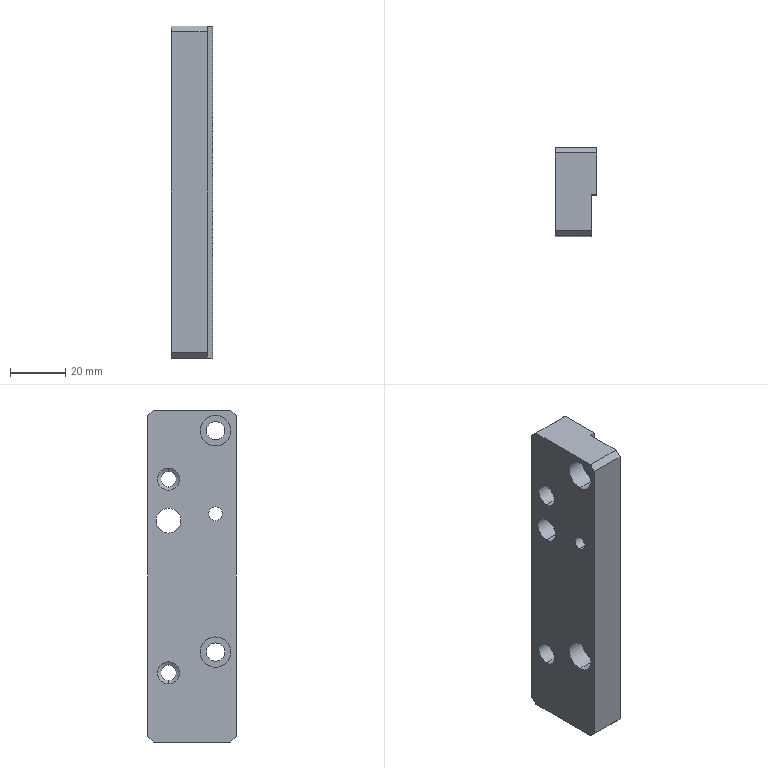Part | SolidWorks | features HoleWzd 5, Chamfer 1, Cut 1, Extrusion 1 | 1 solid | 44 faces | box 15 x 32 x 120 mm | volume 49288 mm3 | cylinder 24 | plane 16 | cone 4 | commonest cylinder face diameters 5.5 x4 6.6 x4 8 x4 10 x4 11 x4 5 x2
STEP:
#1=CARTESIAN_POINT('',(13.,-8.5,20.));
#2=VERTEX_POINT('',#1);
#3=CARTESIAN_POINT('',(13.,-8.5,25.));
#4=VERTEX_POINT('',#3);
#5=CARTESIAN_POINT('',(13.,-8.5,22.5));
#6=DIRECTION('',(-1.,0.,0.));
#7=DIRECTION('',(0.,0.,1.));
#8=AXIS2_PLACEMENT_3D('',#5,#6,#7);
#9=CIRCLE('',#8,2.5);
#10=EDGE_CURVE('',#2,#4,#9,.T.);
#11=ORIENTED_EDGE('',*,*,#10,.F.);
#12=CARTESIAN_POINT('',(0.,-8.5,20.));
#13=VERTEX_POINT('',#12);
#14=CARTESIAN_POINT('',(0.,-8.5,20.));
#15=DIRECTION('',(-1.,0.,0.));
#16=VECTOR('',#15,1000.);
#17=LINE('',#14,#16);
#18=EDGE_CURVE('',#2,#13,#17,.T.);
#19=ORIENTED_EDGE('',*,*,#18,.T.);
#20=CARTESIAN_POINT('',(0.,-8.5,25.));
#21=VERTEX_POINT('',#20);
#22=CARTESIAN_POINT('',(0.,-8.5,22.5));
#23=DIRECTION('',(-1.,0.,0.));
#24=DIRECTION('',(0.,0.,1.));
#25=AXIS2_PLACEMENT_3D('',#22,#23,#24);
#26=CIRCLE('',#25,2.5);
#27=EDGE_CURVE('',#13,#21,#26,.T.);
#28=ORIENTED_EDGE('',*,*,#27,.T.);
#29=CARTESIAN_POINT('',(0.,-8.5,25.));
#30=DIRECTION('',(-1.,0.,0.));
#31=VECTOR('',#30,1000.);
#32=LINE('',#29,#31);
#33=EDGE_CURVE('',#4,#21,#32,.T.);
#34=ORIENTED_EDGE('',*,*,#33,.F.);
#35=EDGE_LOOP('',(#11,#19,#28,#34));
#36=FACE_OUTER_BOUND('',#35,.T.);
#37=CARTESIAN_POINT('',(0.,-8.5,22.5));
#38=DIRECTION('',(-1.,0.,0.));
#39=DIRECTION('',(0.,0.,1.));
#40=AXIS2_PLACEMENT_3D('',#37,#38,#39);
#41=CYLINDRICAL_SURFACE('',#40,2.5);
#42=ADVANCED_FACE('',(#36),#41,.F.);
#43=CARTESIAN_POINT('',(6.8,-8.5,-33.));
#44=VERTEX_POINT('',#43);
#45=CARTESIAN_POINT('',(6.8,-8.5,-22.));
#46=VERTEX_POINT('',#45);
#47=CARTESIAN_POINT('',(6.8,-8.5,-27.5));
#48=DIRECTION('',(-1.,0.,0.));
#49=DIRECTION('',(0.,0.,1.));
#50=AXIS2_PLACEMENT_3D('',#47,#48,#49);
#51=CIRCLE('',#50,5.5);
#52=EDGE_CURVE('',#44,#46,#51,.T.);
#53=ORIENTED_EDGE('',*,*,#52,.F.);
#54=CARTESIAN_POINT('',(0.,-8.5,-33.));
#55=VERTEX_POINT('',#54);
#56=CARTESIAN_POINT('',(0.,-8.5,-33.));
#57=DIRECTION('',(-1.,0.,0.));
#58=VECTOR('',#57,1000.);
#59=LINE('',#56,#58);
#60=EDGE_CURVE('',#44,#55,#59,.T.);
#61=ORIENTED_EDGE('',*,*,#60,.T.);
#62=CARTESIAN_POINT('',(0.,-8.5,-22.));
#63=VERTEX_POINT('',#62);
#64=CARTESIAN_POINT('',(0.,-8.5,-27.5));
#65=DIRECTION('',(-1.,0.,0.));
#66=DIRECTION('',(0.,0.,1.));
#67=AXIS2_PLACEMENT_3D('',#64,#65,#66);
#68=CIRCLE('',#67,5.5);
#69=EDGE_CURVE('',#55,#63,#68,.T.);
#70=ORIENTED_EDGE('',*,*,#69,.T.);
#71=CARTESIAN_POINT('',(0.,-8.5,-22.));
#72=DIRECTION('',(-1.,0.,0.));
#73=VECTOR('',#72,1000.);
#74=LINE('',#71,#73);
#75=EDGE_CURVE('',#46,#63,#74,.T.);
#76=ORIENTED_EDGE('',*,*,#75,.F.);
#77=EDGE_LOOP('',(#53,#61,#70,#76));
#78=FACE_OUTER_BOUND('',#77,.T.);
#79=CARTESIAN_POINT('',(0.,-8.5,-27.5));
#80=DIRECTION('',(-1.,0.,0.));
#81=DIRECTION('',(0.,0.,1.));
#82=AXIS2_PLACEMENT_3D('',#79,#80,#81);
#83=CYLINDRICAL_SURFACE('',#82,5.5);
#84=ADVANCED_FACE('',(#78),#83,.F.);
#85=CARTESIAN_POINT('',(13.,-8.5,-30.8));
#86=VERTEX_POINT('',#85);
#87=CARTESIAN_POINT('',(13.,-8.5,-24.2));
#88=VERTEX_POINT('',#87);
#89=CARTESIAN_POINT('',(13.,-8.5,-27.5));
#90=DIRECTION('',(-1.,0.,0.));
#91=DIRECTION('',(0.,0.,1.));
#92=AXIS2_PLACEMENT_3D('',#89,#90,#91);
#93=CIRCLE('',#92,3.3);
#94=EDGE_CURVE('',#86,#88,#93,.T.);
#95=ORIENTED_EDGE('',*,*,#94,.F.);
#96=CARTESIAN_POINT('',(6.8,-8.5,-30.8));
#97=VERTEX_POINT('',#96);
#98=CARTESIAN_POINT('',(0.,-8.5,-30.8));
#99=DIRECTION('',(-1.,0.,0.));
#100=VECTOR('',#99,1000.);
#101=LINE('',#98,#100);
#102=EDGE_CURVE('',#86,#97,#101,.T.);
#103=ORIENTED_EDGE('',*,*,#102,.T.);
#104=CARTESIAN_POINT('',(6.8,-8.5,-24.2));
#105=VERTEX_POINT('',#104);
#106=CARTESIAN_POINT('',(6.8,-8.5,-27.5));
#107=DIRECTION('',(-1.,0.,0.));
#108=DIRECTION('',(0.,0.,1.));
#109=AXIS2_PLACEMENT_3D('',#106,#107,#108);
#110=CIRCLE('',#109,3.3);
#111=EDGE_CURVE('',#97,#105,#110,.T.);
#112=ORIENTED_EDGE('',*,*,#111,.T.);
#113=CARTESIAN_POINT('',(0.,-8.5,-24.2));
#114=DIRECTION('',(-1.,0.,0.));
#115=VECTOR('',#114,1000.);
#116=LINE('',#113,#115);
#117=EDGE_CURVE('',#88,#105,#116,.T.);
#118=ORIENTED_EDGE('',*,*,#117,.F.);
#119=EDGE_LOOP('',(#95,#103,#112,#118));
#120=FACE_OUTER_BOUND('',#119,.T.);
#121=CARTESIAN_POINT('',(0.,-8.5,-27.5));
#122=DIRECTION('',(-1.,0.,0.));
#123=DIRECTION('',(0.,0.,1.));
#124=AXIS2_PLACEMENT_3D('',#121,#122,#123);
#125=CYLINDRICAL_SURFACE('',#124,3.3);
#126=ADVANCED_FACE('',(#120),#125,.F.);
#127=CARTESIAN_POINT('',(6.8,-8.5,47.));
#128=VERTEX_POINT('',#127);
#129=CARTESIAN_POINT('',(6.8,-8.5,58.));
#130=VERTEX_POINT('',#129);
#131=CARTESIAN_POINT('',(6.8,-8.5,52.5));
#132=DIRECTION('',(-1.,0.,0.));
#133=DIRECTION('',(0.,0.,1.));
#134=AXIS2_PLACEMENT_3D('',#131,#132,#133);
#135=CIRCLE('',#134,5.5);
#136=EDGE_CURVE('',#128,#130,#135,.T.);
#137=ORIENTED_EDGE('',*,*,#136,.F.);
#138=CARTESIAN_POINT('',(0.,-8.5,47.));
#139=VERTEX_POINT('',#138);
#140=CARTESIAN_POINT('',(0.,-8.5,47.));
#141=DIRECTION('',(-1.,0.,0.));
#142=VECTOR('',#141,1000.);
#143=LINE('',#140,#142);
#144=EDGE_CURVE('',#128,#139,#143,.T.);
#145=ORIENTED_EDGE('',*,*,#144,.T.);
#146=CARTESIAN_POINT('',(0.,-8.5,58.));
#147=VERTEX_POINT('',#146);
#148=CARTESIAN_POINT('',(0.,-8.5,52.5));
#149=DIRECTION('',(-1.,0.,0.));
#150=DIRECTION('',(0.,0.,1.));
#151=AXIS2_PLACEMENT_3D('',#148,#149,#150);
#152=CIRCLE('',#151,5.5);
#153=EDGE_CURVE('',#139,#147,#152,.T.);
#154=ORIENTED_EDGE('',*,*,#153,.T.);
#155=CARTESIAN_POINT('',(0.,-8.5,58.));
#156=DIRECTION('',(-1.,0.,0.));
#157=VECTOR('',#156,1000.);
#158=LINE('',#155,#157);
#159=EDGE_CURVE('',#130,#147,#158,.T.);
#160=ORIENTED_EDGE('',*,*,#159,.F.);
#161=EDGE_LOOP('',(#137,#145,#154,#160));
#162=FACE_OUTER_BOUND('',#161,.T.);
#163=CARTESIAN_POINT('',(0.,-8.5,52.5));
#164=DIRECTION('',(-1.,0.,0.));
#165=DIRECTION('',(0.,0.,1.));
#166=AXIS2_PLACEMENT_3D('',#163,#164,#165);
#167=CYLINDRICAL_SURFACE('',#166,5.5);
#168=ADVANCED_FACE('',(#162),#167,.F.);
#169=CARTESIAN_POINT('',(13.,-8.5,49.2));
#170=VERTEX_POINT('',#169);
#171=CARTESIAN_POINT('',(13.,-8.5,55.8));
#172=VERTEX_POINT('',#171);
#173=CARTESIAN_POINT('',(13.,-8.5,52.5));
#174=DIRECTION('',(-1.,0.,0.));
#175=DIRECTION('',(0.,0.,1.));
#176=AXIS2_PLACEMENT_3D('',#173,#174,#175);
#177=CIRCLE('',#176,3.3);
#178=EDGE_CURVE('',#170,#172,#177,.T.);
#179=ORIENTED_EDGE('',*,*,#178,.F.);
#180=CARTESIAN_POINT('',(6.8,-8.5,49.2));
#181=VERTEX_POINT('',#180);
#182=CARTESIAN_POINT('',(0.,-8.5,49.2));
#183=DIRECTION('',(-1.,0.,0.));
#184=VECTOR('',#183,1000.);
#185=LINE('',#182,#184);
#186=EDGE_CURVE('',#170,#181,#185,.T.);
#187=ORIENTED_EDGE('',*,*,#186,.T.);
#188=CARTESIAN_POINT('',(6.8,-8.5,55.8));
#189=VERTEX_POINT('',#188);
#190=CARTESIAN_POINT('',(6.8,-8.5,52.5));
#191=DIRECTION('',(-1.,0.,0.));
#192=DIRECTION('',(0.,0.,1.));
#193=AXIS2_PLACEMENT_3D('',#190,#191,#192);
#194=CIRCLE('',#193,3.3);
#195=EDGE_CURVE('',#181,#189,#194,.T.);
#196=ORIENTED_EDGE('',*,*,#195,.T.);
#197=CARTESIAN_POINT('',(0.,-8.5,55.8));
#198=DIRECTION('',(-1.,0.,0.));
#199=VECTOR('',#198,1000.);
#200=LINE('',#197,#199);
#201=EDGE_CURVE('',#172,#189,#200,.T.);
#202=ORIENTED_EDGE('',*,*,#201,.F.);
#203=EDGE_LOOP('',(#179,#187,#196,#202));
#204=FACE_OUTER_BOUND('',#203,.T.);
#205=CARTESIAN_POINT('',(0.,-8.5,52.5));
#206=DIRECTION('',(-1.,0.,0.));
#207=DIRECTION('',(0.,0.,1.));
#208=AXIS2_PLACEMENT_3D('',#205,#206,#207);
#209=CYLINDRICAL_SURFACE('',#208,3.3);
#210=ADVANCED_FACE('',(#204),#209,.F.);
#211=CARTESIAN_POINT('',(9.3,8.5,40.));
#212=VERTEX_POINT('',#211);
#213=CARTESIAN_POINT('',(9.3,8.5,30.));
#214=VERTEX_POINT('',#213);
#215=CARTESIAN_POINT('',(9.3,8.5,35.));
#216=DIRECTION('',(1.,0.,0.));
#217=DIRECTION('',(0.,0.,-1.));
#218=AXIS2_PLACEMENT_3D('',#215,#216,#217);
#219=CIRCLE('',#218,5.);
#220=EDGE_CURVE('',#212,#214,#219,.T.);
#221=ORIENTED_EDGE('',*,*,#220,.F.);
#222=CARTESIAN_POINT('',(15.,8.5,40.));
#223=VERTEX_POINT('',#222);
#224=CARTESIAN_POINT('',(15.,8.5,40.));
#225=DIRECTION('',(1.,0.,0.));
#226=VECTOR('',#225,1000.);
#227=LINE('',#224,#226);
#228=EDGE_CURVE('',#212,#223,#227,.T.);
#229=ORIENTED_EDGE('',*,*,#228,.T.);
#230=CARTESIAN_POINT('',(15.,8.5,30.));
#231=VERTEX_POINT('',#230);
#232=CARTESIAN_POINT('',(15.,8.5,35.));
#233=DIRECTION('',(1.,0.,0.));
#234=DIRECTION('',(0.,0.,-1.));
#235=AXIS2_PLACEMENT_3D('',#232,#233,#234);
#236=CIRCLE('',#235,5.);
#237=EDGE_CURVE('',#223,#231,#236,.T.);
#238=ORIENTED_EDGE('',*,*,#237,.T.);
#239=CARTESIAN_POINT('',(15.,8.5,30.));
#240=DIRECTION('',(1.,0.,0.));
#241=VECTOR('',#240,1000.);
#242=LINE('',#239,#241);
#243=EDGE_CURVE('',#214,#231,#242,.T.);
#244=ORIENTED_EDGE('',*,*,#243,.F.);
#245=EDGE_LOOP('',(#221,#229,#238,#244));
#246=FACE_OUTER_BOUND('',#245,.T.);
#247=CARTESIAN_POINT('',(15.,8.5,35.));
#248=DIRECTION('',(1.,0.,0.));
#249=DIRECTION('',(0.,0.,-1.));
#250=AXIS2_PLACEMENT_3D('',#247,#248,#249);
#251=CYLINDRICAL_SURFACE('',#250,5.);
#252=ADVANCED_FACE('',(#246),#251,.F.);
#253=CARTESIAN_POINT('',(6.751,8.5,37.75));
#254=VERTEX_POINT('',#253);
#255=CARTESIAN_POINT('',(6.751,8.5,32.25));
#256=VERTEX_POINT('',#255);
#257=CARTESIAN_POINT('',(6.751,8.5,35.));
#258=DIRECTION('',(1.,0.,0.));
#259=DIRECTION('',(0.,0.,1.));
#260=AXIS2_PLACEMENT_3D('',#257,#258,#259);
#261=CIRCLE('',#260,2.75);
#262=EDGE_CURVE('',#254,#256,#261,.T.);
#263=ORIENTED_EDGE('',*,*,#262,.F.);
#264=CARTESIAN_POINT('',(9.3,8.5,37.75));
#265=VERTEX_POINT('',#264);
#266=CARTESIAN_POINT('',(15.,8.5,37.75));
#267=DIRECTION('',(1.,0.,0.));
#268=VECTOR('',#267,1000.);
#269=LINE('',#266,#268);
#270=EDGE_CURVE('',#254,#265,#269,.T.);
#271=ORIENTED_EDGE('',*,*,#270,.T.);
#272=CARTESIAN_POINT('',(9.3,8.5,32.25));
#273=VERTEX_POINT('',#272);
#274=CARTESIAN_POINT('',(9.3,8.5,35.));
#275=DIRECTION('',(1.,0.,0.));
#276=DIRECTION('',(0.,0.,-1.));
#277=AXIS2_PLACEMENT_3D('',#274,#275,#276);
#278=CIRCLE('',#277,2.75);
#279=EDGE_CURVE('',#265,#273,#278,.T.);
#280=ORIENTED_EDGE('',*,*,#279,.T.);
#281=CARTESIAN_POINT('',(15.,8.5,32.25));
#282=DIRECTION('',(1.,0.,0.));
#283=VECTOR('',#282,1000.);
#284=LINE('',#281,#283);
#285=EDGE_CURVE('',#256,#273,#284,.T.);
#286=ORIENTED_EDGE('',*,*,#285,.F.);
#287=EDGE_LOOP('',(#263,#271,#280,#286));
#288=FACE_OUTER_BOUND('',#287,.T.);
#289=CARTESIAN_POINT('',(15.,8.5,35.));
#290=DIRECTION('',(1.,0.,0.));
#291=DIRECTION('',(0.,0.,-1.));
#292=AXIS2_PLACEMENT_3D('',#289,#290,#291);
#293=CYLINDRICAL_SURFACE('',#292,2.75);
#294=ADVANCED_FACE('',(#288),#293,.F.);
#295=CARTESIAN_POINT('',(9.3,8.5,-30.));
#296=VERTEX_POINT('',#295);
#297=CARTESIAN_POINT('',(9.3,8.5,-40.));
#298=VERTEX_POINT('',#297);
#299=CARTESIAN_POINT('',(9.3,8.5,-35.));
#300=DIRECTION('',(1.,0.,0.));
#301=DIRECTION('',(0.,0.,-1.));
#302=AXIS2_PLACEMENT_3D('',#299,#300,#301);
#303=CIRCLE('',#302,5.);
#304=EDGE_CURVE('',#296,#298,#303,.T.);
#305=ORIENTED_EDGE('',*,*,#304,.F.);
#306=CARTESIAN_POINT('',(15.,8.5,-30.));
#307=VERTEX_POINT('',#306);
#308=CARTESIAN_POINT('',(15.,8.5,-30.));
#309=DIRECTION('',(1.,0.,0.));
#310=VECTOR('',#309,1000.);
#311=LINE('',#308,#310);
#312=EDGE_CURVE('',#296,#307,#311,.T.);
#313=ORIENTED_EDGE('',*,*,#312,.T.);
#314=CARTESIAN_POINT('',(15.,8.5,-40.));
#315=VERTEX_POINT('',#314);
#316=CARTESIAN_POINT('',(15.,8.5,-35.));
#317=DIRECTION('',(1.,0.,0.));
#318=DIRECTION('',(0.,0.,-1.));
#319=AXIS2_PLACEMENT_3D('',#316,#317,#318);
#320=CIRCLE('',#319,5.);
#321=EDGE_CURVE('',#307,#315,#320,.T.);
#322=ORIENTED_EDGE('',*,*,#321,.T.);
#323=CARTESIAN_POINT('',(15.,8.5,-40.));
#324=DIRECTION('',(1.,0.,0.));
#325=VECTOR('',#324,1000.);
#326=LINE('',#323,#325);
#327=EDGE_CURVE('',#298,#315,#326,.T.);
#328=ORIENTED_EDGE('',*,*,#327,.F.);
#329=EDGE_LOOP('',(#305,#313,#322,#328));
#330=FACE_OUTER_BOUND('',#329,.T.);
#331=CARTESIAN_POINT('',(15.,8.5,-35.));
#332=DIRECTION('',(1.,0.,0.));
#333=DIRECTION('',(0.,0.,-1.));
#334=AXIS2_PLACEMENT_3D('',#331,#332,#333);
#335=CYLINDRICAL_SURFACE('',#334,5.);
#336=ADVANCED_FACE('',(#330),#335,.F.);
#337=CARTESIAN_POINT('',(6.751,8.5,-32.25));
#338=VERTEX_POINT('',#337);
#339=CARTESIAN_POINT('',(6.751,8.5,-37.75));
#340=VERTEX_POINT('',#339);
#341=CARTESIAN_POINT('',(6.751,8.5,-35.));
#342=DIRECTION('',(1.,0.,0.));
#343=DIRECTION('',(0.,0.,1.));
#344=AXIS2_PLACEMENT_3D('',#341,#342,#343);
#345=CIRCLE('',#344,2.75);
#346=EDGE_CURVE('',#338,#340,#345,.T.);
#347=ORIENTED_EDGE('',*,*,#346,.F.);
#348=CARTESIAN_POINT('',(9.3,8.5,-32.25));
#349=VERTEX_POINT('',#348);
#350=CARTESIAN_POINT('',(15.,8.5,-32.25));
#351=DIRECTION('',(1.,0.,0.));
#352=VECTOR('',#351,1000.);
#353=LINE('',#350,#352);
#354=EDGE_CURVE('',#338,#349,#353,.T.);
#355=ORIENTED_EDGE('',*,*,#354,.T.);
#356=CARTESIAN_POINT('',(9.3,8.5,-37.75));
#357=VERTEX_POINT('',#356);
#358=CARTESIAN_POINT('',(9.3,8.5,-35.));
#359=DIRECTION('',(1.,0.,0.));
#360=DIRECTION('',(0.,0.,-1.));
#361=AXIS2_PLACEMENT_3D('',#358,#359,#360);
#362=CIRCLE('',#361,2.75);
#363=EDGE_CURVE('',#349,#357,#362,.T.);
#364=ORIENTED_EDGE('',*,*,#363,.T.);
#365=CARTESIAN_POINT('',(15.,8.5,-37.75));
#366=DIRECTION('',(1.,0.,0.));
#367=VECTOR('',#366,1000.);
#368=LINE('',#365,#367);
#369=EDGE_CURVE('',#340,#357,#368,.T.);
#370=ORIENTED_EDGE('',*,*,#369,.F.);
#371=EDGE_LOOP('',(#347,#355,#364,#370));
#372=FACE_OUTER_BOUND('',#371,.T.);
#373=CARTESIAN_POINT('',(15.,8.5,-35.));
#374=DIRECTION('',(1.,0.,0.));
#375=DIRECTION('',(0.,0.,-1.));
#376=AXIS2_PLACEMENT_3D('',#373,#374,#375);
#377=CYLINDRICAL_SURFACE('',#376,2.75);
#378=ADVANCED_FACE('',(#372),#377,.F.);
#379=CARTESIAN_POINT('',(0.,8.5,24.5));
#380=VERTEX_POINT('',#379);
#381=CARTESIAN_POINT('',(0.,8.5,15.5));
#382=VERTEX_POINT('',#381);
#383=CARTESIAN_POINT('',(0.,8.5,20.));
#384=DIRECTION('',(1.,0.,0.));
#385=DIRECTION('',(0.,0.,-1.));
#386=AXIS2_PLACEMENT_3D('',#383,#384,#385);
#387=CIRCLE('',#386,4.5);
#388=EDGE_CURVE('',#380,#382,#387,.T.);
#389=ORIENTED_EDGE('',*,*,#388,.F.);
#390=CARTESIAN_POINT('',(15.,8.5,24.5));
#391=VERTEX_POINT('',#390);
#392=CARTESIAN_POINT('',(15.,8.5,24.5));
#393=DIRECTION('',(1.,0.,0.));
#394=VECTOR('',#393,1000.);
#395=LINE('',#392,#394);
#396=EDGE_CURVE('',#380,#391,#395,.T.);
#397=ORIENTED_EDGE('',*,*,#396,.T.);
#398=CARTESIAN_POINT('',(15.,8.5,15.5));
#399=VERTEX_POINT('',#398);
#400=CARTESIAN_POINT('',(15.,8.5,20.));
#401=DIRECTION('',(1.,0.,0.));
#402=DIRECTION('',(0.,0.,-1.));
#403=AXIS2_PLACEMENT_3D('',#400,#401,#402);
#404=CIRCLE('',#403,4.5);
#405=EDGE_CURVE('',#391,#399,#404,.T.);
#406=ORIENTED_EDGE('',*,*,#405,.T.);
#407=CARTESIAN_POINT('',(15.,8.5,15.5));
#408=DIRECTION('',(1.,0.,0.));
#409=VECTOR('',#408,1000.);
#410=LINE('',#407,#409);
#411=EDGE_CURVE('',#382,#399,#410,.T.);
#412=ORIENTED_EDGE('',*,*,#411,.F.);
#413=EDGE_LOOP('',(#389,#397,#406,#412));
#414=FACE_OUTER_BOUND('',#413,.T.);
#415=CARTESIAN_POINT('',(15.,8.5,20.));
#416=DIRECTION('',(1.,0.,0.));
#417=DIRECTION('',(0.,0.,-1.));
#418=AXIS2_PLACEMENT_3D('',#415,#416,#417);
#419=CYLINDRICAL_SURFACE('',#418,4.5);
#420=ADVANCED_FACE('',(#414),#419,.F.);
#421=CARTESIAN_POINT('',(6.,8.5,31.));
#422=VERTEX_POINT('',#421);
#423=CARTESIAN_POINT('',(6.,8.5,39.));
#424=VERTEX_POINT('',#423);
#425=CARTESIAN_POINT('',(6.,8.5,35.));
#426=DIRECTION('',(-1.,0.,0.));
#427=DIRECTION('',(0.,0.,1.));
#428=AXIS2_PLACEMENT_3D('',#425,#426,#427);
#429=CIRCLE('',#428,4.);
#430=EDGE_CURVE('',#422,#424,#429,.T.);
#431=ORIENTED_EDGE('',*,*,#430,.F.);
#432=CARTESIAN_POINT('',(0.,8.5,31.));
#433=VERTEX_POINT('',#432);
#434=CARTESIAN_POINT('',(0.,8.5,31.));
#435=DIRECTION('',(-1.,0.,0.));
#436=VECTOR('',#435,1000.);
#437=LINE('',#434,#436);
#438=EDGE_CURVE('',#422,#433,#437,.T.);
#439=ORIENTED_EDGE('',*,*,#438,.T.);
#440=CARTESIAN_POINT('',(0.,8.5,39.));
#441=VERTEX_POINT('',#440);
#442=CARTESIAN_POINT('',(0.,8.5,35.));
#443=DIRECTION('',(-1.,0.,0.));
#444=DIRECTION('',(0.,0.,1.));
#445=AXIS2_PLACEMENT_3D('',#442,#443,#444);
#446=CIRCLE('',#445,4.);
#447=EDGE_CURVE('',#433,#441,#446,.T.);
#448=ORIENTED_EDGE('',*,*,#447,.T.);
#449=CARTESIAN_POINT('',(0.,8.5,39.));
#450=DIRECTION('',(-1.,0.,0.));
#451=VECTOR('',#450,1000.);
#452=LINE('',#449,#451);
#453=EDGE_CURVE('',#424,#441,#452,.T.);
#454=ORIENTED_EDGE('',*,*,#453,.F.);
#455=EDGE_LOOP('',(#431,#439,#448,#454));
#456=FACE_OUTER_BOUND('',#455,.T.);
#457=CARTESIAN_POINT('',(0.,8.5,35.));
#458=DIRECTION('',(-1.,0.,0.));
#459=DIRECTION('',(0.,0.,1.));
#460=AXIS2_PLACEMENT_3D('',#457,#458,#459);
#461=CYLINDRICAL_SURFACE('',#460,4.);
#462=ADVANCED_FACE('',(#456),#461,.F.);
#463=ORIENTED_EDGE('',*,*,#262,.T.);
#464=CARTESIAN_POINT('',(6.,8.5,31.));
#465=DIRECTION('',(-0.515,0.,-0.8572));
#466=VECTOR('',#465,1000.);
#467=LINE('',#464,#466);
#468=EDGE_CURVE('',#256,#422,#467,.T.);
#469=ORIENTED_EDGE('',*,*,#468,.T.);
#470=ORIENTED_EDGE('',*,*,#430,.T.);
#471=CARTESIAN_POINT('',(6.,8.5,39.));
#472=DIRECTION('',(-0.515,0.,0.8572));
#473=VECTOR('',#472,1000.);
#474=LINE('',#471,#473);
#475=EDGE_CURVE('',#254,#424,#474,.T.);
#476=ORIENTED_EDGE('',*,*,#475,.F.);
#477=EDGE_LOOP('',(#463,#469,#470,#476));
#478=FACE_OUTER_BOUND('',#477,.T.);
#479=CARTESIAN_POINT('',(6.,8.5,35.));
#480=DIRECTION('',(-1.,0.,0.));
#481=DIRECTION('',(0.,0.,1.));
#482=AXIS2_PLACEMENT_3D('',#479,#480,#481);
#483=CONICAL_SURFACE('',#482,4.,1.03);
#484=ADVANCED_FACE('',(#478),#483,.F.);
#485=CARTESIAN_POINT('',(6.,8.5,-39.));
#486=VERTEX_POINT('',#485);
#487=CARTESIAN_POINT('',(6.,8.5,-31.));
#488=VERTEX_POINT('',#487);
#489=CARTESIAN_POINT('',(6.,8.5,-35.));
#490=DIRECTION('',(-1.,0.,0.));
#491=DIRECTION('',(0.,0.,1.));
#492=AXIS2_PLACEMENT_3D('',#489,#490,#491);
#493=CIRCLE('',#492,4.);
#494=EDGE_CURVE('',#486,#488,#493,.T.);
#495=ORIENTED_EDGE('',*,*,#494,.F.);
#496=CARTESIAN_POINT('',(0.,8.5,-39.));
#497=VERTEX_POINT('',#496);
#498=CARTESIAN_POINT('',(0.,8.5,-39.));
#499=DIRECTION('',(-1.,0.,0.));
#500=VECTOR('',#499,1000.);
#501=LINE('',#498,#500);
#502=EDGE_CURVE('',#486,#497,#501,.T.);
#503=ORIENTED_EDGE('',*,*,#502,.T.);
#504=CARTESIAN_POINT('',(0.,8.5,-31.));
#505=VERTEX_POINT('',#504);
#506=CARTESIAN_POINT('',(0.,8.5,-35.));
#507=DIRECTION('',(-1.,0.,0.));
#508=DIRECTION('',(0.,0.,1.));
#509=AXIS2_PLACEMENT_3D('',#506,#507,#508);
#510=CIRCLE('',#509,4.);
#511=EDGE_CURVE('',#497,#505,#510,.T.);
#512=ORIENTED_EDGE('',*,*,#511,.T.);
#513=CARTESIAN_POINT('',(0.,8.5,-31.));
#514=DIRECTION('',(-1.,0.,0.));
#515=VECTOR('',#514,1000.);
#516=LINE('',#513,#515);
#517=EDGE_CURVE('',#488,#505,#516,.T.);
#518=ORIENTED_EDGE('',*,*,#517,.F.);
#519=EDGE_LOOP('',(#495,#503,#512,#518));
#520=FACE_OUTER_BOUND('',#519,.T.);
#521=CARTESIAN_POINT('',(0.,8.5,-35.));
#522=DIRECTION('',(-1.,0.,0.));
#523=DIRECTION('',(0.,0.,1.));
#524=AXIS2_PLACEMENT_3D('',#521,#522,#523);
#525=CYLINDRICAL_SURFACE('',#524,4.);
#526=ADVANCED_FACE('',(#520),#525,.F.);
#527=ORIENTED_EDGE('',*,*,#346,.T.);
#528=CARTESIAN_POINT('',(6.,8.5,-39.));
#529=DIRECTION('',(-0.515,0.,-0.8572));
#530=VECTOR('',#529,1000.);
#531=LINE('',#528,#530);
#532=EDGE_CURVE('',#340,#486,#531,.T.);
#533=ORIENTED_EDGE('',*,*,#532,.T.);
#534=ORIENTED_EDGE('',*,*,#494,.T.);
#535=CARTESIAN_POINT('',(6.,8.5,-31.));
#536=DIRECTION('',(-0.515,0.,0.8572));
#537=VECTOR('',#536,1000.);
#538=LINE('',#535,#537);
#539=EDGE_CURVE('',#338,#488,#538,.T.);
#540=ORIENTED_EDGE('',*,*,#539,.F.);
#541=EDGE_LOOP('',(#527,#533,#534,#540));
#542=FACE_OUTER_BOUND('',#541,.T.);
#543=CARTESIAN_POINT('',(6.,8.5,-35.));
#544=DIRECTION('',(-1.,0.,0.));
#545=DIRECTION('',(0.,0.,1.));
#546=AXIS2_PLACEMENT_3D('',#543,#544,#545);
#547=CONICAL_SURFACE('',#546,4.,1.03);
#548=ADVANCED_FACE('',(#542),#547,.F.);
#549=CARTESIAN_POINT('',(13.,-14.,-60.));
#550=VERTEX_POINT('',#549);
#551=CARTESIAN_POINT('',(13.,-1.,-60.));
#552=VERTEX_POINT('',#551);
#553=CARTESIAN_POINT('',(13.,-16.,-60.));
#554=DIRECTION('',(0.,1.,0.));
#555=VECTOR('',#554,1000.);
#556=LINE('',#553,#555);
#557=EDGE_CURVE('',#550,#552,#556,.T.);
#558=ORIENTED_EDGE('',*,*,#557,.F.);
#559=CARTESIAN_POINT('',(0.,-14.,-60.));
#560=VERTEX_POINT('',#559);
#561=CARTESIAN_POINT('',(15.,-14.,-60.));
#562=DIRECTION('',(-1.,0.,0.));
#563=VECTOR('',#562,1000.);
#564=LINE('',#561,#563);
#565=EDGE_CURVE('',#550,#560,#564,.T.);
#566=ORIENTED_EDGE('',*,*,#565,.T.);
#567=CARTESIAN_POINT('',(0.,14.,-60.));
#568=VERTEX_POINT('',#567);
#569=CARTESIAN_POINT('',(0.,-16.,-60.));
#570=DIRECTION('',(0.,1.,0.));
#571=VECTOR('',#570,1000.);
#572=LINE('',#569,#571);
#573=EDGE_CURVE('',#560,#568,#572,.T.);
#574=ORIENTED_EDGE('',*,*,#573,.T.);
#575=CARTESIAN_POINT('',(15.,14.,-60.));
#576=VERTEX_POINT('',#575);
#577=CARTESIAN_POINT('',(15.,14.,-60.));
#578=DIRECTION('',(1.,0.,0.));
#579=VECTOR('',#578,1000.);
#580=LINE('',#577,#579);
#581=EDGE_CURVE('',#568,#576,#580,.T.);
#582=ORIENTED_EDGE('',*,*,#581,.T.);
#583=CARTESIAN_POINT('',(15.,-1.,-60.));
#584=VERTEX_POINT('',#583);
#585=CARTESIAN_POINT('',(15.,-16.,-60.));
#586=DIRECTION('',(0.,1.,0.));
#587=VECTOR('',#586,1000.);
#588=LINE('',#585,#587);
#589=EDGE_CURVE('',#584,#576,#588,.T.);
#590=ORIENTED_EDGE('',*,*,#589,.F.);
#591=CARTESIAN_POINT('',(13.,-1.,-60.));
#592=DIRECTION('',(1.,0.,0.));
#593=VECTOR('',#592,1000.);
#594=LINE('',#591,#593);
#595=EDGE_CURVE('',#552,#584,#594,.T.);
#596=ORIENTED_EDGE('',*,*,#595,.F.);
#597=EDGE_LOOP('',(#558,#566,#574,#582,#590,#596));
#598=FACE_OUTER_BOUND('',#597,.T.);
#599=CARTESIAN_POINT('',(15.,-16.,-60.));
#600=DIRECTION('',(0.,0.,1.));
#601=DIRECTION('',(1.,0.,0.));
#602=AXIS2_PLACEMENT_3D('',#599,#600,#601);
#603=PLANE('',#602);
#604=ADVANCED_FACE('',(#598),#603,.F.);
#605=CARTESIAN_POINT('',(15.,16.,-58.));
#606=VERTEX_POINT('',#605);
#607=CARTESIAN_POINT('',(15.,16.,58.));
#608=VERTEX_POINT('',#607);
#609=CARTESIAN_POINT('',(15.,16.,60.));
#610=DIRECTION('',(0.,0.,1.));
#611=VECTOR('',#610,1000.);
#612=LINE('',#609,#611);
#613=EDGE_CURVE('',#606,#608,#612,.T.);
#614=ORIENTED_EDGE('',*,*,#613,.F.);
#615=CARTESIAN_POINT('',(0.,16.,-58.));
#616=VERTEX_POINT('',#615);
#617=CARTESIAN_POINT('',(15.,16.,-58.));
#618=DIRECTION('',(-1.,0.,0.));
#619=VECTOR('',#618,1000.);
#620=LINE('',#617,#619);
#621=EDGE_CURVE('',#606,#616,#620,.T.);
#622=ORIENTED_EDGE('',*,*,#621,.T.);
#623=CARTESIAN_POINT('',(0.,16.,58.));
#624=VERTEX_POINT('',#623);
#625=CARTESIAN_POINT('',(0.,16.,60.));
#626=DIRECTION('',(0.,0.,1.));
#627=VECTOR('',#626,1000.);
#628=LINE('',#625,#627);
#629=EDGE_CURVE('',#616,#624,#628,.T.);
#630=ORIENTED_EDGE('',*,*,#629,.T.);
#631=CARTESIAN_POINT('',(15.,16.,58.));
#632=DIRECTION('',(1.,0.,0.));
#633=VECTOR('',#632,1000.);
#634=LINE('',#631,#633);
#635=EDGE_CURVE('',#624,#608,#634,.T.);
#636=ORIENTED_EDGE('',*,*,#635,.T.);
#637=EDGE_LOOP('',(#614,#622,#630,#636));
#638=FACE_OUTER_BOUND('',#637,.T.);
#639=CARTESIAN_POINT('',(15.,16.,60.));
#640=DIRECTION('',(0.,-1.,0.));
#641=DIRECTION('',(0.,0.,-1.));
#642=AXIS2_PLACEMENT_3D('',#639,#640,#641);
#643=PLANE('',#642);
#644=ADVANCED_FACE('',(#638),#643,.F.);
#645=CARTESIAN_POINT('',(0.,14.,60.));
#646=VERTEX_POINT('',#645);
#647=CARTESIAN_POINT('',(0.,-14.,60.));
#648=VERTEX_POINT('',#647);
#649=CARTESIAN_POINT('',(0.,-16.,60.));
#650=DIRECTION('',(0.,-1.,0.));
#651=VECTOR('',#650,1000.);
#652=LINE('',#649,#651);
#653=EDGE_CURVE('',#646,#648,#652,.T.);
#654=ORIENTED_EDGE('',*,*,#653,.T.);
#655=CARTESIAN_POINT('',(13.,-14.,60.));
#656=VERTEX_POINT('',#655);
#657=CARTESIAN_POINT('',(15.,-14.,60.));
#658=DIRECTION('',(1.,0.,0.));
#659=VECTOR('',#658,1000.);
#660=LINE('',#657,#659);
#661=EDGE_CURVE('',#648,#656,#660,.T.);
#662=ORIENTED_EDGE('',*,*,#661,.T.);
#663=CARTESIAN_POINT('',(13.,-1.,60.));
#664=VERTEX_POINT('',#663);
#665=CARTESIAN_POINT('',(13.,-16.,60.));
#666=DIRECTION('',(0.,-1.,0.));
#667=VECTOR('',#666,1000.);
#668=LINE('',#665,#667);
#669=EDGE_CURVE('',#664,#656,#668,.T.);
#670=ORIENTED_EDGE('',*,*,#669,.F.);
#671=CARTESIAN_POINT('',(15.,-1.,60.));
#672=VERTEX_POINT('',#671);
#673=CARTESIAN_POINT('',(13.,-1.,60.));
#674=DIRECTION('',(1.,0.,0.));
#675=VECTOR('',#674,1000.);
#676=LINE('',#673,#675);
#677=EDGE_CURVE('',#664,#672,#676,.T.);
#678=ORIENTED_EDGE('',*,*,#677,.T.);
#679=CARTESIAN_POINT('',(15.,14.,60.));
#680=VERTEX_POINT('',#679);
#681=CARTESIAN_POINT('',(15.,-16.,60.));
#682=DIRECTION('',(0.,-1.,0.));
#683=VECTOR('',#682,1000.);
#684=LINE('',#681,#683);
#685=EDGE_CURVE('',#680,#672,#684,.T.);
#686=ORIENTED_EDGE('',*,*,#685,.F.);
#687=CARTESIAN_POINT('',(15.,14.,60.));
#688=DIRECTION('',(-1.,0.,0.));
#689=VECTOR('',#688,1000.);
#690=LINE('',#687,#689);
#691=EDGE_CURVE('',#680,#646,#690,.T.);
#692=ORIENTED_EDGE('',*,*,#691,.T.);
#693=EDGE_LOOP('',(#654,#662,#670,#678,#686,#692));
#694=FACE_OUTER_BOUND('',#693,.T.);
#695=CARTESIAN_POINT('',(15.,-16.,60.));
#696=DIRECTION('',(0.,0.,-1.));
#697=DIRECTION('',(-1.,0.,0.));
#698=AXIS2_PLACEMENT_3D('',#695,#696,#697);
#699=PLANE('',#698);
#700=ADVANCED_FACE('',(#694),#699,.F.);
#701=CARTESIAN_POINT('',(0.,-16.,58.));
#702=VERTEX_POINT('',#701);
#703=CARTESIAN_POINT('',(0.,-16.,-58.));
#704=VERTEX_POINT('',#703);
#705=CARTESIAN_POINT('',(0.,-16.,60.));
#706=DIRECTION('',(0.,0.,-1.));
#707=VECTOR('',#706,1000.);
#708=LINE('',#705,#707);
#709=EDGE_CURVE('',#702,#704,#708,.T.);
#710=ORIENTED_EDGE('',*,*,#709,.T.);
#711=CARTESIAN_POINT('',(13.,-16.,-58.));
#712=VERTEX_POINT('',#711);
#713=CARTESIAN_POINT('',(15.,-16.,-58.));
#714=DIRECTION('',(1.,0.,0.));
#715=VECTOR('',#714,1000.);
#716=LINE('',#713,#715);
#717=EDGE_CURVE('',#704,#712,#716,.T.);
#718=ORIENTED_EDGE('',*,*,#717,.T.);
#719=CARTESIAN_POINT('',(13.,-16.,58.));
#720=VERTEX_POINT('',#719);
#721=CARTESIAN_POINT('',(13.,-16.,60.));
#722=DIRECTION('',(0.,0.,-1.));
#723=VECTOR('',#722,1000.);
#724=LINE('',#721,#723);
#725=EDGE_CURVE('',#720,#712,#724,.T.);
#726=ORIENTED_EDGE('',*,*,#725,.F.);
#727=CARTESIAN_POINT('',(15.,-16.,58.));
#728=DIRECTION('',(-1.,0.,0.));
#729=VECTOR('',#728,1000.);
#730=LINE('',#727,#729);
#731=EDGE_CURVE('',#720,#702,#730,.T.);
#732=ORIENTED_EDGE('',*,*,#731,.T.);
#733=EDGE_LOOP('',(#710,#718,#726,#732));
#734=FACE_OUTER_BOUND('',#733,.T.);
#735=CARTESIAN_POINT('',(15.,-16.,60.));
#736=DIRECTION('',(0.,1.,0.));
#737=DIRECTION('',(0.,0.,1.));
#738=AXIS2_PLACEMENT_3D('',#735,#736,#737);
#739=PLANE('',#738);
#740=ADVANCED_FACE('',(#734),#739,.F.);
#741=CARTESIAN_POINT('',(15.,8.5,35.));
#742=DIRECTION('',(1.,0.,0.));
#743=DIRECTION('',(0.,0.,-1.));
#744=AXIS2_PLACEMENT_3D('',#741,#742,#743);
#745=CIRCLE('',#744,5.);
#746=EDGE_CURVE('',#231,#223,#745,.T.);
#747=ORIENTED_EDGE('',*,*,#746,.F.);
#748=ORIENTED_EDGE('',*,*,#237,.F.);
#749=EDGE_LOOP('',(#747,#748));
#750=FACE_BOUND('',#749,.T.);
#751=CARTESIAN_POINT('',(15.,8.5,-35.));
#752=DIRECTION('',(1.,0.,0.));
#753=DIRECTION('',(0.,0.,-1.));
#754=AXIS2_PLACEMENT_3D('',#751,#752,#753);
#755=CIRCLE('',#754,5.);
#756=EDGE_CURVE('',#315,#307,#755,.T.);
#757=ORIENTED_EDGE('',*,*,#756,.F.);
#758=ORIENTED_EDGE('',*,*,#321,.F.);
#759=EDGE_LOOP('',(#757,#758));
#760=FACE_BOUND('',#759,.T.);
#761=CARTESIAN_POINT('',(15.,8.5,20.));
#762=DIRECTION('',(1.,0.,0.));
#763=DIRECTION('',(0.,0.,-1.));
#764=AXIS2_PLACEMENT_3D('',#761,#762,#763);
#765=CIRCLE('',#764,4.5);
#766=EDGE_CURVE('',#399,#391,#765,.T.);
#767=ORIENTED_EDGE('',*,*,#766,.F.);
#768=ORIENTED_EDGE('',*,*,#405,.F.);
#769=EDGE_LOOP('',(#767,#768));
#770=FACE_BOUND('',#769,.T.);
#771=ORIENTED_EDGE('',*,*,#589,.T.);
#772=CARTESIAN_POINT('',(15.,16.,-58.));
#773=DIRECTION('',(0.,0.7071,0.7071));
#774=VECTOR('',#773,1000.);
#775=LINE('',#772,#774);
#776=EDGE_CURVE('',#576,#606,#775,.T.);
#777=ORIENTED_EDGE('',*,*,#776,.T.);
#778=ORIENTED_EDGE('',*,*,#613,.T.);
#779=CARTESIAN_POINT('',(15.,14.,60.));
#780=DIRECTION('',(0.,-0.7071,0.7071));
#781=VECTOR('',#780,1000.);
#782=LINE('',#779,#781);
#783=EDGE_CURVE('',#608,#680,#782,.T.);
#784=ORIENTED_EDGE('',*,*,#783,.T.);
#785=ORIENTED_EDGE('',*,*,#685,.T.);
#786=CARTESIAN_POINT('',(15.,-1.,60.));
#787=DIRECTION('',(0.,0.,1.));
#788=VECTOR('',#787,1000.);
#789=LINE('',#786,#788);
#790=EDGE_CURVE('',#584,#672,#789,.T.);
#791=ORIENTED_EDGE('',*,*,#790,.F.);
#792=EDGE_LOOP('',(#771,#777,#778,#784,#785,#791));
#793=FACE_OUTER_BOUND('',#792,.T.);
#794=CARTESIAN_POINT('',(15.,0.,0.));
#795=DIRECTION('',(-1.,0.,0.));
#796=DIRECTION('',(0.,0.,1.));
#797=AXIS2_PLACEMENT_3D('',#794,#795,#796);
#798=PLANE('',#797);
#799=ADVANCED_FACE('',(#750,#760,#770,#793),#798,.F.);
#800=CARTESIAN_POINT('',(0.,-8.5,22.5));
#801=DIRECTION('',(-1.,0.,0.));
#802=DIRECTION('',(0.,0.,1.));
#803=AXIS2_PLACEMENT_3D('',#800,#801,#802);
#804=CIRCLE('',#803,2.5);
#805=EDGE_CURVE('',#21,#13,#804,.T.);
#806=ORIENTED_EDGE('',*,*,#805,.F.);
#807=ORIENTED_EDGE('',*,*,#27,.F.);
#808=EDGE_LOOP('',(#806,#807));
#809=FACE_BOUND('',#808,.T.);
#810=CARTESIAN_POINT('',(0.,-8.5,-27.5));
#811=DIRECTION('',(-1.,0.,0.));
#812=DIRECTION('',(0.,0.,1.));
#813=AXIS2_PLACEMENT_3D('',#810,#811,#812);
#814=CIRCLE('',#813,5.5);
#815=EDGE_CURVE('',#63,#55,#814,.T.);
#816=ORIENTED_EDGE('',*,*,#815,.F.);
#817=ORIENTED_EDGE('',*,*,#69,.F.);
#818=EDGE_LOOP('',(#816,#817));
#819=FACE_BOUND('',#818,.T.);
#820=CARTESIAN_POINT('',(0.,-8.5,52.5));
#821=DIRECTION('',(-1.,0.,0.));
#822=DIRECTION('',(0.,0.,1.));
#823=AXIS2_PLACEMENT_3D('',#820,#821,#822);
#824=CIRCLE('',#823,5.5);
#825=EDGE_CURVE('',#147,#139,#824,.T.);
#826=ORIENTED_EDGE('',*,*,#825,.F.);
#827=ORIENTED_EDGE('',*,*,#153,.F.);
#828=EDGE_LOOP('',(#826,#827));
#829=FACE_BOUND('',#828,.T.);
#830=CARTESIAN_POINT('',(0.,8.5,20.));
#831=DIRECTION('',(1.,0.,0.));
#832=DIRECTION('',(0.,0.,-1.));
#833=AXIS2_PLACEMENT_3D('',#830,#831,#832);
#834=CIRCLE('',#833,4.5);
#835=EDGE_CURVE('',#382,#380,#834,.T.);
#836=ORIENTED_EDGE('',*,*,#835,.T.);
#837=ORIENTED_EDGE('',*,*,#388,.T.);
#838=EDGE_LOOP('',(#836,#837));
#839=FACE_BOUND('',#838,.T.);
#840=CARTESIAN_POINT('',(0.,8.5,35.));
#841=DIRECTION('',(-1.,0.,0.));
#842=DIRECTION('',(0.,0.,1.));
#843=AXIS2_PLACEMENT_3D('',#840,#841,#842);
#844=CIRCLE('',#843,4.);
#845=EDGE_CURVE('',#441,#433,#844,.T.);
#846=ORIENTED_EDGE('',*,*,#845,.F.);
#847=ORIENTED_EDGE('',*,*,#447,.F.);
#848=EDGE_LOOP('',(#846,#847));
#849=FACE_BOUND('',#848,.T.);
#850=CARTESIAN_POINT('',(0.,8.5,-35.));
#851=DIRECTION('',(-1.,0.,0.));
#852=DIRECTION('',(0.,0.,1.));
#853=AXIS2_PLACEMENT_3D('',#850,#851,#852);
#854=CIRCLE('',#853,4.);
#855=EDGE_CURVE('',#505,#497,#854,.T.);
#856=ORIENTED_EDGE('',*,*,#855,.F.);
#857=ORIENTED_EDGE('',*,*,#511,.F.);
#858=EDGE_LOOP('',(#856,#857));
#859=FACE_BOUND('',#858,.T.);
#860=ORIENTED_EDGE('',*,*,#573,.F.);
#861=CARTESIAN_POINT('',(0.,-37.,-37.));
#862=DIRECTION('',(0.,-0.7071,0.7071));
#863=VECTOR('',#862,1000.);
#864=LINE('',#861,#863);
#865=EDGE_CURVE('',#560,#704,#864,.T.);
#866=ORIENTED_EDGE('',*,*,#865,.T.);
#867=ORIENTED_EDGE('',*,*,#709,.F.);
#868=CARTESIAN_POINT('',(0.,-37.,37.));
#869=DIRECTION('',(0.,0.7071,0.7071));
#870=VECTOR('',#869,1000.);
#871=LINE('',#868,#870);
#872=EDGE_CURVE('',#702,#648,#871,.T.);
#873=ORIENTED_EDGE('',*,*,#872,.T.);
#874=ORIENTED_EDGE('',*,*,#653,.F.);
#875=CARTESIAN_POINT('',(0.,37.,37.));
#876=DIRECTION('',(0.,0.7071,-0.7071));
#877=VECTOR('',#876,1000.);
#878=LINE('',#875,#877);
#879=EDGE_CURVE('',#646,#624,#878,.T.);
#880=ORIENTED_EDGE('',*,*,#879,.T.);
#881=ORIENTED_EDGE('',*,*,#629,.F.);
#882=CARTESIAN_POINT('',(0.,37.,-37.));
#883=DIRECTION('',(0.,-0.7071,-0.7071));
#884=VECTOR('',#883,1000.);
#885=LINE('',#882,#884);
#886=EDGE_CURVE('',#616,#568,#885,.T.);
#887=ORIENTED_EDGE('',*,*,#886,.T.);
#888=EDGE_LOOP('',(#860,#866,#867,#873,#874,#880,#881,#887));
#889=FACE_OUTER_BOUND('',#888,.T.);
#890=CARTESIAN_POINT('',(0.,0.,0.));
#891=DIRECTION('',(-1.,0.,0.));
#892=DIRECTION('',(0.,0.,1.));
#893=AXIS2_PLACEMENT_3D('',#890,#891,#892);
#894=PLANE('',#893);
#895=ADVANCED_FACE('',(#809,#819,#829,#839,#849,#859,#889),#894,.T.);
#896=ORIENTED_EDGE('',*,*,#790,.T.);
#897=ORIENTED_EDGE('',*,*,#677,.F.);
#898=CARTESIAN_POINT('',(13.,-1.,60.));
#899=DIRECTION('',(0.,0.,1.));
#900=VECTOR('',#899,1000.);
#901=LINE('',#898,#900);
#902=EDGE_CURVE('',#552,#664,#901,.T.);
#903=ORIENTED_EDGE('',*,*,#902,.F.);
#904=ORIENTED_EDGE('',*,*,#595,.T.);
#905=EDGE_LOOP('',(#896,#897,#903,#904));
#906=FACE_OUTER_BOUND('',#905,.T.);
#907=CARTESIAN_POINT('',(13.,-1.,60.));
#908=DIRECTION('',(0.,1.,0.));
#909=DIRECTION('',(0.,0.,1.));
#910=AXIS2_PLACEMENT_3D('',#907,#908,#909);
#911=PLANE('',#910);
#912=ADVANCED_FACE('',(#906),#911,.F.);
#913=CARTESIAN_POINT('',(13.,-8.5,22.5));
#914=DIRECTION('',(-1.,0.,0.));
#915=DIRECTION('',(0.,0.,1.));
#916=AXIS2_PLACEMENT_3D('',#913,#914,#915);
#917=CIRCLE('',#916,2.5);
#918=EDGE_CURVE('',#4,#2,#917,.T.);
#919=ORIENTED_EDGE('',*,*,#918,.T.);
#920=ORIENTED_EDGE('',*,*,#10,.T.);
#921=EDGE_LOOP('',(#919,#920));
#922=FACE_BOUND('',#921,.T.);
#923=CARTESIAN_POINT('',(13.,-8.5,-27.5));
#924=DIRECTION('',(-1.,0.,0.));
#925=DIRECTION('',(0.,0.,1.));
#926=AXIS2_PLACEMENT_3D('',#923,#924,#925);
#927=CIRCLE('',#926,3.3);
#928=EDGE_CURVE('',#88,#86,#927,.T.);
#929=ORIENTED_EDGE('',*,*,#928,.T.);
#930=ORIENTED_EDGE('',*,*,#94,.T.);
#931=EDGE_LOOP('',(#929,#930));
#932=FACE_BOUND('',#931,.T.);
#933=CARTESIAN_POINT('',(13.,-8.5,52.5));
#934=DIRECTION('',(-1.,0.,0.));
#935=DIRECTION('',(0.,0.,1.));
#936=AXIS2_PLACEMENT_3D('',#933,#934,#935);
#937=CIRCLE('',#936,3.3);
#938=EDGE_CURVE('',#172,#170,#937,.T.);
#939=ORIENTED_EDGE('',*,*,#938,.T.);
#940=ORIENTED_EDGE('',*,*,#178,.T.);
#941=EDGE_LOOP('',(#939,#940));
#942=FACE_BOUND('',#941,.T.);
#943=ORIENTED_EDGE('',*,*,#725,.T.);
#944=CARTESIAN_POINT('',(13.,-14.,-60.));
#945=DIRECTION('',(0.,0.7071,-0.7071));
#946=VECTOR('',#945,1000.);
#947=LINE('',#944,#946);
#948=EDGE_CURVE('',#712,#550,#947,.T.);
#949=ORIENTED_EDGE('',*,*,#948,.T.);
#950=ORIENTED_EDGE('',*,*,#557,.T.);
#951=ORIENTED_EDGE('',*,*,#902,.T.);
#952=ORIENTED_EDGE('',*,*,#669,.T.);
#953=CARTESIAN_POINT('',(13.,-16.,58.));
#954=DIRECTION('',(0.,-0.7071,-0.7071));
#955=VECTOR('',#954,1000.);
#956=LINE('',#953,#955);
#957=EDGE_CURVE('',#656,#720,#956,.T.);
#958=ORIENTED_EDGE('',*,*,#957,.T.);
#959=EDGE_LOOP('',(#943,#949,#950,#951,#952,#958));
#960=FACE_OUTER_BOUND('',#959,.T.);
#961=CARTESIAN_POINT('',(13.,0.,0.));
#962=DIRECTION('',(-1.,0.,0.));
#963=DIRECTION('',(0.,0.,1.));
#964=AXIS2_PLACEMENT_3D('',#961,#962,#963);
#965=PLANE('',#964);
#966=ADVANCED_FACE('',(#922,#932,#942,#960),#965,.F.);
#967=ORIENTED_EDGE('',*,*,#532,.F.);
#968=CARTESIAN_POINT('',(6.751,8.5,-35.));
#969=DIRECTION('',(1.,0.,0.));
#970=DIRECTION('',(0.,0.,1.));
#971=AXIS2_PLACEMENT_3D('',#968,#969,#970);
#972=CIRCLE('',#971,2.75);
#973=EDGE_CURVE('',#340,#338,#972,.T.);
#974=ORIENTED_EDGE('',*,*,#973,.T.);
#975=ORIENTED_EDGE('',*,*,#539,.T.);
#976=CARTESIAN_POINT('',(6.,8.5,-35.));
#977=DIRECTION('',(-1.,0.,0.));
#978=DIRECTION('',(0.,0.,1.));
#979=AXIS2_PLACEMENT_3D('',#976,#977,#978);
#980=CIRCLE('',#979,4.);
#981=EDGE_CURVE('',#488,#486,#980,.T.);
#982=ORIENTED_EDGE('',*,*,#981,.T.);
#983=EDGE_LOOP('',(#967,#974,#975,#982));
#984=FACE_OUTER_BOUND('',#983,.T.);
#985=CARTESIAN_POINT('',(6.,8.5,-35.));
#986=DIRECTION('',(-1.,0.,0.));
#987=DIRECTION('',(0.,0.,1.));
#988=AXIS2_PLACEMENT_3D('',#985,#986,#987);
#989=CONICAL_SURFACE('',#988,4.,1.03);
#990=ADVANCED_FACE('',(#984),#989,.F.);
#991=ORIENTED_EDGE('',*,*,#502,.F.);
#992=ORIENTED_EDGE('',*,*,#981,.F.);
#993=ORIENTED_EDGE('',*,*,#517,.T.);
#994=ORIENTED_EDGE('',*,*,#855,.T.);
#995=EDGE_LOOP('',(#991,#992,#993,#994));
#996=FACE_OUTER_BOUND('',#995,.T.);
#997=CARTESIAN_POINT('',(0.,8.5,-35.));
#998=DIRECTION('',(-1.,0.,0.));
#999=DIRECTION('',(0.,0.,1.));
#1000=AXIS2_PLACEMENT_3D('',#997,#998,#999);
#1001=CYLINDRICAL_SURFACE('',#1000,4.);
#1002=ADVANCED_FACE('',(#996),#1001,.F.);
#1003=ORIENTED_EDGE('',*,*,#468,.F.);
#1004=CARTESIAN_POINT('',(6.751,8.5,35.));
#1005=DIRECTION('',(1.,0.,0.));
#1006=DIRECTION('',(0.,0.,1.));
#1007=AXIS2_PLACEMENT_3D('',#1004,#1005,#1006);
#1008=CIRCLE('',#1007,2.75);
#1009=EDGE_CURVE('',#256,#254,#1008,.T.);
#1010=ORIENTED_EDGE('',*,*,#1009,.T.);
#1011=ORIENTED_EDGE('',*,*,#475,.T.);
#1012=CARTESIAN_POINT('',(6.,8.5,35.));
#1013=DIRECTION('',(-1.,0.,0.));
#1014=DIRECTION('',(0.,0.,1.));
#1015=AXIS2_PLACEMENT_3D('',#1012,#1013,#1014);
#1016=CIRCLE('',#1015,4.);
#1017=EDGE_CURVE('',#424,#422,#1016,.T.);
#1018=ORIENTED_EDGE('',*,*,#1017,.T.);
#1019=EDGE_LOOP('',(#1003,#1010,#1011,#1018));
#1020=FACE_OUTER_BOUND('',#1019,.T.);
#1021=CARTESIAN_POINT('',(6.,8.5,35.));
#1022=DIRECTION('',(-1.,0.,0.));
#1023=DIRECTION('',(0.,0.,1.));
#1024=AXIS2_PLACEMENT_3D('',#1021,#1022,#1023);
#1025=CONICAL_SURFACE('',#1024,4.,1.03);
#1026=ADVANCED_FACE('',(#1020),#1025,.F.);
#1027=ORIENTED_EDGE('',*,*,#438,.F.);
#1028=ORIENTED_EDGE('',*,*,#1017,.F.);
#1029=ORIENTED_EDGE('',*,*,#453,.T.);
#1030=ORIENTED_EDGE('',*,*,#845,.T.);
#1031=EDGE_LOOP('',(#1027,#1028,#1029,#1030));
#1032=FACE_OUTER_BOUND('',#1031,.T.);
#1033=CARTESIAN_POINT('',(0.,8.5,35.));
#1034=DIRECTION('',(-1.,0.,0.));
#1035=DIRECTION('',(0.,0.,1.));
#1036=AXIS2_PLACEMENT_3D('',#1033,#1034,#1035);
#1037=CYLINDRICAL_SURFACE('',#1036,4.);
#1038=ADVANCED_FACE('',(#1032),#1037,.F.);
#1039=ORIENTED_EDGE('',*,*,#396,.F.);
#1040=ORIENTED_EDGE('',*,*,#835,.F.);
#1041=ORIENTED_EDGE('',*,*,#411,.T.);
#1042=ORIENTED_EDGE('',*,*,#766,.T.);
#1043=EDGE_LOOP('',(#1039,#1040,#1041,#1042));
#1044=FACE_OUTER_BOUND('',#1043,.T.);
#1045=CARTESIAN_POINT('',(15.,8.5,20.));
#1046=DIRECTION('',(1.,0.,0.));
#1047=DIRECTION('',(0.,0.,-1.));
#1048=AXIS2_PLACEMENT_3D('',#1045,#1046,#1047);
#1049=CYLINDRICAL_SURFACE('',#1048,4.5);
#1050=ADVANCED_FACE('',(#1044),#1049,.F.);
#1051=ORIENTED_EDGE('',*,*,#948,.F.);
#1052=ORIENTED_EDGE('',*,*,#717,.F.);
#1053=ORIENTED_EDGE('',*,*,#865,.F.);
#1054=ORIENTED_EDGE('',*,*,#565,.F.);
#1055=EDGE_LOOP('',(#1051,#1052,#1053,#1054));
#1056=FACE_OUTER_BOUND('',#1055,.T.);
#1057=CARTESIAN_POINT('',(15.,-14.,-60.));
#1058=DIRECTION('',(0.,0.7071,0.7071));
#1059=DIRECTION('',(-1.,0.,0.));
#1060=AXIS2_PLACEMENT_3D('',#1057,#1058,#1059);
#1061=PLANE('',#1060);
#1062=ADVANCED_FACE('',(#1056),#1061,.F.);
#1063=ORIENTED_EDGE('',*,*,#776,.F.);
#1064=ORIENTED_EDGE('',*,*,#581,.F.);
#1065=ORIENTED_EDGE('',*,*,#886,.F.);
#1066=ORIENTED_EDGE('',*,*,#621,.F.);
#1067=EDGE_LOOP('',(#1063,#1064,#1065,#1066));
#1068=FACE_OUTER_BOUND('',#1067,.T.);
#1069=CARTESIAN_POINT('',(15.,16.,-58.));
#1070=DIRECTION('',(0.,-0.7071,0.7071));
#1071=DIRECTION('',(-1.,0.,0.));
#1072=AXIS2_PLACEMENT_3D('',#1069,#1070,#1071);
#1073=PLANE('',#1072);
#1074=ADVANCED_FACE('',(#1068),#1073,.F.);
#1075=ORIENTED_EDGE('',*,*,#957,.F.);
#1076=ORIENTED_EDGE('',*,*,#661,.F.);
#1077=ORIENTED_EDGE('',*,*,#872,.F.);
#1078=ORIENTED_EDGE('',*,*,#731,.F.);
#1079=EDGE_LOOP('',(#1075,#1076,#1077,#1078));
#1080=FACE_OUTER_BOUND('',#1079,.T.);
#1081=CARTESIAN_POINT('',(15.,-16.,58.));
#1082=DIRECTION('',(0.,0.7071,-0.7071));
#1083=DIRECTION('',(-1.,0.,0.));
#1084=AXIS2_PLACEMENT_3D('',#1081,#1082,#1083);
#1085=PLANE('',#1084);
#1086=ADVANCED_FACE('',(#1080),#1085,.F.);
#1087=ORIENTED_EDGE('',*,*,#783,.F.);
#1088=ORIENTED_EDGE('',*,*,#635,.F.);
#1089=ORIENTED_EDGE('',*,*,#879,.F.);
#1090=ORIENTED_EDGE('',*,*,#691,.F.);
#1091=EDGE_LOOP('',(#1087,#1088,#1089,#1090));
#1092=FACE_OUTER_BOUND('',#1091,.T.);
#1093=CARTESIAN_POINT('',(15.,14.,60.));
#1094=DIRECTION('',(0.,-0.7071,-0.7071));
#1095=DIRECTION('',(-1.,0.,0.));
#1096=AXIS2_PLACEMENT_3D('',#1093,#1094,#1095);
#1097=PLANE('',#1096);
#1098=ADVANCED_FACE('',(#1092),#1097,.F.);
#1099=ORIENTED_EDGE('',*,*,#354,.F.);
#1100=ORIENTED_EDGE('',*,*,#973,.F.);
#1101=ORIENTED_EDGE('',*,*,#369,.T.);
#1102=CARTESIAN_POINT('',(9.3,8.5,-35.));
#1103=DIRECTION('',(1.,0.,0.));
#1104=DIRECTION('',(0.,0.,-1.));
#1105=AXIS2_PLACEMENT_3D('',#1102,#1103,#1104);
#1106=CIRCLE('',#1105,2.75);
#1107=EDGE_CURVE('',#357,#349,#1106,.T.);
#1108=ORIENTED_EDGE('',*,*,#1107,.T.);
#1109=EDGE_LOOP('',(#1099,#1100,#1101,#1108));
#1110=FACE_OUTER_BOUND('',#1109,.T.);
#1111=CARTESIAN_POINT('',(15.,8.5,-35.));
#1112=DIRECTION('',(1.,0.,0.));
#1113=DIRECTION('',(0.,0.,-1.));
#1114=AXIS2_PLACEMENT_3D('',#1111,#1112,#1113);
#1115=CYLINDRICAL_SURFACE('',#1114,2.75);
#1116=ADVANCED_FACE('',(#1110),#1115,.F.);
#1117=ORIENTED_EDGE('',*,*,#1107,.F.);
#1118=ORIENTED_EDGE('',*,*,#363,.F.);
#1119=EDGE_LOOP('',(#1117,#1118));
#1120=FACE_BOUND('',#1119,.T.);
#1121=CARTESIAN_POINT('',(9.3,8.5,-35.));
#1122=DIRECTION('',(1.,0.,0.));
#1123=DIRECTION('',(0.,0.,-1.));
#1124=AXIS2_PLACEMENT_3D('',#1121,#1122,#1123);
#1125=CIRCLE('',#1124,5.);
#1126=EDGE_CURVE('',#298,#296,#1125,.T.);
#1127=ORIENTED_EDGE('',*,*,#1126,.T.);
#1128=ORIENTED_EDGE('',*,*,#304,.T.);
#1129=EDGE_LOOP('',(#1127,#1128));
#1130=FACE_OUTER_BOUND('',#1129,.T.);
#1131=CARTESIAN_POINT('',(9.3,11.25,-35.));
#1132=DIRECTION('',(-1.,0.,0.));
#1133=DIRECTION('',(0.,0.,1.));
#1134=AXIS2_PLACEMENT_3D('',#1131,#1132,#1133);
#1135=PLANE('',#1134);
#1136=ADVANCED_FACE('',(#1120,#1130),#1135,.F.);
#1137=ORIENTED_EDGE('',*,*,#312,.F.);
#1138=ORIENTED_EDGE('',*,*,#1126,.F.);
#1139=ORIENTED_EDGE('',*,*,#327,.T.);
#1140=ORIENTED_EDGE('',*,*,#756,.T.);
#1141=EDGE_LOOP('',(#1137,#1138,#1139,#1140));
#1142=FACE_OUTER_BOUND('',#1141,.T.);
#1143=CARTESIAN_POINT('',(15.,8.5,-35.));
#1144=DIRECTION('',(1.,0.,0.));
#1145=DIRECTION('',(0.,0.,-1.));
#1146=AXIS2_PLACEMENT_3D('',#1143,#1144,#1145);
#1147=CYLINDRICAL_SURFACE('',#1146,5.);
#1148=ADVANCED_FACE('',(#1142),#1147,.F.);
#1149=ORIENTED_EDGE('',*,*,#270,.F.);
#1150=ORIENTED_EDGE('',*,*,#1009,.F.);
#1151=ORIENTED_EDGE('',*,*,#285,.T.);
#1152=CARTESIAN_POINT('',(9.3,8.5,35.));
#1153=DIRECTION('',(1.,0.,0.));
#1154=DIRECTION('',(0.,0.,-1.));
#1155=AXIS2_PLACEMENT_3D('',#1152,#1153,#1154);
#1156=CIRCLE('',#1155,2.75);
#1157=EDGE_CURVE('',#273,#265,#1156,.T.);
#1158=ORIENTED_EDGE('',*,*,#1157,.T.);
#1159=EDGE_LOOP('',(#1149,#1150,#1151,#1158));
#1160=FACE_OUTER_BOUND('',#1159,.T.);
#1161=CARTESIAN_POINT('',(15.,8.5,35.));
#1162=DIRECTION('',(1.,0.,0.));
#1163=DIRECTION('',(0.,0.,-1.));
#1164=AXIS2_PLACEMENT_3D('',#1161,#1162,#1163);
#1165=CYLINDRICAL_SURFACE('',#1164,2.75);
#1166=ADVANCED_FACE('',(#1160),#1165,.F.);
#1167=ORIENTED_EDGE('',*,*,#1157,.F.);
#1168=ORIENTED_EDGE('',*,*,#279,.F.);
#1169=EDGE_LOOP('',(#1167,#1168));
#1170=FACE_BOUND('',#1169,.T.);
#1171=CARTESIAN_POINT('',(9.3,8.5,35.));
#1172=DIRECTION('',(1.,0.,0.));
#1173=DIRECTION('',(0.,0.,-1.));
#1174=AXIS2_PLACEMENT_3D('',#1171,#1172,#1173);
#1175=CIRCLE('',#1174,5.);
#1176=EDGE_CURVE('',#214,#212,#1175,.T.);
#1177=ORIENTED_EDGE('',*,*,#1176,.T.);
#1178=ORIENTED_EDGE('',*,*,#220,.T.);
#1179=EDGE_LOOP('',(#1177,#1178));
#1180=FACE_OUTER_BOUND('',#1179,.T.);
#1181=CARTESIAN_POINT('',(9.3,11.25,35.));
#1182=DIRECTION('',(-1.,0.,0.));
#1183=DIRECTION('',(0.,0.,1.));
#1184=AXIS2_PLACEMENT_3D('',#1181,#1182,#1183);
#1185=PLANE('',#1184);
#1186=ADVANCED_FACE('',(#1170,#1180),#1185,.F.);
#1187=ORIENTED_EDGE('',*,*,#228,.F.);
#1188=ORIENTED_EDGE('',*,*,#1176,.F.);
#1189=ORIENTED_EDGE('',*,*,#243,.T.);
#1190=ORIENTED_EDGE('',*,*,#746,.T.);
#1191=EDGE_LOOP('',(#1187,#1188,#1189,#1190));
#1192=FACE_OUTER_BOUND('',#1191,.T.);
#1193=CARTESIAN_POINT('',(15.,8.5,35.));
#1194=DIRECTION('',(1.,0.,0.));
#1195=DIRECTION('',(0.,0.,-1.));
#1196=AXIS2_PLACEMENT_3D('',#1193,#1194,#1195);
#1197=CYLINDRICAL_SURFACE('',#1196,5.);
#1198=ADVANCED_FACE('',(#1192),#1197,.F.);
#1199=ORIENTED_EDGE('',*,*,#186,.F.);
#1200=ORIENTED_EDGE('',*,*,#938,.F.);
#1201=ORIENTED_EDGE('',*,*,#201,.T.);
#1202=CARTESIAN_POINT('',(6.8,-8.5,52.5));
#1203=DIRECTION('',(-1.,0.,0.));
#1204=DIRECTION('',(0.,0.,1.));
#1205=AXIS2_PLACEMENT_3D('',#1202,#1203,#1204);
#1206=CIRCLE('',#1205,3.3);
#1207=EDGE_CURVE('',#189,#181,#1206,.T.);
#1208=ORIENTED_EDGE('',*,*,#1207,.T.);
#1209=EDGE_LOOP('',(#1199,#1200,#1201,#1208));
#1210=FACE_OUTER_BOUND('',#1209,.T.);
#1211=CARTESIAN_POINT('',(0.,-8.5,52.5));
#1212=DIRECTION('',(-1.,0.,0.));
#1213=DIRECTION('',(0.,0.,1.));
#1214=AXIS2_PLACEMENT_3D('',#1211,#1212,#1213);
#1215=CYLINDRICAL_SURFACE('',#1214,3.3);
#1216=ADVANCED_FACE('',(#1210),#1215,.F.);
#1217=ORIENTED_EDGE('',*,*,#1207,.F.);
#1218=ORIENTED_EDGE('',*,*,#195,.F.);
#1219=EDGE_LOOP('',(#1217,#1218));
#1220=FACE_BOUND('',#1219,.T.);
#1221=CARTESIAN_POINT('',(6.8,-8.5,52.5));
#1222=DIRECTION('',(-1.,0.,0.));
#1223=DIRECTION('',(0.,0.,1.));
#1224=AXIS2_PLACEMENT_3D('',#1221,#1222,#1223);
#1225=CIRCLE('',#1224,5.5);
#1226=EDGE_CURVE('',#130,#128,#1225,.T.);
#1227=ORIENTED_EDGE('',*,*,#1226,.T.);
#1228=ORIENTED_EDGE('',*,*,#136,.T.);
#1229=EDGE_LOOP('',(#1227,#1228));
#1230=FACE_OUTER_BOUND('',#1229,.T.);
#1231=CARTESIAN_POINT('',(6.8,-5.2,52.5));
#1232=DIRECTION('',(1.,0.,0.));
#1233=DIRECTION('',(0.,0.,-1.));
#1234=AXIS2_PLACEMENT_3D('',#1231,#1232,#1233);
#1235=PLANE('',#1234);
#1236=ADVANCED_FACE('',(#1220,#1230),#1235,.F.);
#1237=ORIENTED_EDGE('',*,*,#144,.F.);
#1238=ORIENTED_EDGE('',*,*,#1226,.F.);
#1239=ORIENTED_EDGE('',*,*,#159,.T.);
#1240=ORIENTED_EDGE('',*,*,#825,.T.);
#1241=EDGE_LOOP('',(#1237,#1238,#1239,#1240));
#1242=FACE_OUTER_BOUND('',#1241,.T.);
#1243=CARTESIAN_POINT('',(0.,-8.5,52.5));
#1244=DIRECTION('',(-1.,0.,0.));
#1245=DIRECTION('',(0.,0.,1.));
#1246=AXIS2_PLACEMENT_3D('',#1243,#1244,#1245);
#1247=CYLINDRICAL_SURFACE('',#1246,5.5);
#1248=ADVANCED_FACE('',(#1242),#1247,.F.);
#1249=ORIENTED_EDGE('',*,*,#102,.F.);
#1250=ORIENTED_EDGE('',*,*,#928,.F.);
#1251=ORIENTED_EDGE('',*,*,#117,.T.);
#1252=CARTESIAN_POINT('',(6.8,-8.5,-27.5));
#1253=DIRECTION('',(-1.,0.,0.));
#1254=DIRECTION('',(0.,0.,1.));
#1255=AXIS2_PLACEMENT_3D('',#1252,#1253,#1254);
#1256=CIRCLE('',#1255,3.3);
#1257=EDGE_CURVE('',#105,#97,#1256,.T.);
#1258=ORIENTED_EDGE('',*,*,#1257,.T.);
#1259=EDGE_LOOP('',(#1249,#1250,#1251,#1258));
#1260=FACE_OUTER_BOUND('',#1259,.T.);
#1261=CARTESIAN_POINT('',(0.,-8.5,-27.5));
#1262=DIRECTION('',(-1.,0.,0.));
#1263=DIRECTION('',(0.,0.,1.));
#1264=AXIS2_PLACEMENT_3D('',#1261,#1262,#1263);
#1265=CYLINDRICAL_SURFACE('',#1264,3.3);
#1266=ADVANCED_FACE('',(#1260),#1265,.F.);
#1267=ORIENTED_EDGE('',*,*,#1257,.F.);
#1268=ORIENTED_EDGE('',*,*,#111,.F.);
#1269=EDGE_LOOP('',(#1267,#1268));
#1270=FACE_BOUND('',#1269,.T.);
#1271=CARTESIAN_POINT('',(6.8,-8.5,-27.5));
#1272=DIRECTION('',(-1.,0.,0.));
#1273=DIRECTION('',(0.,0.,1.));
#1274=AXIS2_PLACEMENT_3D('',#1271,#1272,#1273);
#1275=CIRCLE('',#1274,5.5);
#1276=EDGE_CURVE('',#46,#44,#1275,.T.);
#1277=ORIENTED_EDGE('',*,*,#1276,.T.);
#1278=ORIENTED_EDGE('',*,*,#52,.T.);
#1279=EDGE_LOOP('',(#1277,#1278));
#1280=FACE_OUTER_BOUND('',#1279,.T.);
#1281=CARTESIAN_POINT('',(6.8,-5.2,-27.5));
#1282=DIRECTION('',(1.,0.,0.));
#1283=DIRECTION('',(0.,0.,-1.));
#1284=AXIS2_PLACEMENT_3D('',#1281,#1282,#1283);
#1285=PLANE('',#1284);
#1286=ADVANCED_FACE('',(#1270,#1280),#1285,.F.);
#1287=ORIENTED_EDGE('',*,*,#60,.F.);
#1288=ORIENTED_EDGE('',*,*,#1276,.F.);
#1289=ORIENTED_EDGE('',*,*,#75,.T.);
#1290=ORIENTED_EDGE('',*,*,#815,.T.);
#1291=EDGE_LOOP('',(#1287,#1288,#1289,#1290));
#1292=FACE_OUTER_BOUND('',#1291,.T.);
#1293=CARTESIAN_POINT('',(0.,-8.5,-27.5));
#1294=DIRECTION('',(-1.,0.,0.));
#1295=DIRECTION('',(0.,0.,1.));
#1296=AXIS2_PLACEMENT_3D('',#1293,#1294,#1295);
#1297=CYLINDRICAL_SURFACE('',#1296,5.5);
#1298=ADVANCED_FACE('',(#1292),#1297,.F.);
#1299=ORIENTED_EDGE('',*,*,#18,.F.);
#1300=ORIENTED_EDGE('',*,*,#918,.F.);
#1301=ORIENTED_EDGE('',*,*,#33,.T.);
#1302=ORIENTED_EDGE('',*,*,#805,.T.);
#1303=EDGE_LOOP('',(#1299,#1300,#1301,#1302));
#1304=FACE_OUTER_BOUND('',#1303,.T.);
#1305=CARTESIAN_POINT('',(0.,-8.5,22.5));
#1306=DIRECTION('',(-1.,0.,0.));
#1307=DIRECTION('',(0.,0.,1.));
#1308=AXIS2_PLACEMENT_3D('',#1305,#1306,#1307);
#1309=CYLINDRICAL_SURFACE('',#1308,2.5);
#1310=ADVANCED_FACE('',(#1304),#1309,.F.);
#1311=CLOSED_SHELL('',(#42,#84,#126,#168,#210,#252,#294,#336,#378,#420,#462,#484,#526,#548,#604,#644,#700,#740,#799,#895,#912,#966,#990,#1002,#1026,#1038,#1050,#1062,#1074,#1086,#1098,#1116,#1136,#1148,#1166,#1186,#1198,#1216,#1236,#1248,#1266,#1286,#1298,#1310));
#1312=MANIFOLD_SOLID_BREP('',#1311);
#1313=CARTESIAN_POINT('',(0.,0.,0.));
#1314=DIRECTION('',(0.,0.,1.));
#1315=DIRECTION('',(1.,0.,0.));
#1316=AXIS2_PLACEMENT_3D('',#1313,#1314,#1315);
#1317=(LENGTH_UNIT()NAMED_UNIT(*)SI_UNIT(.MILLI.,.METRE.));
#1318=UNCERTAINTY_MEASURE_WITH_UNIT(LENGTH_MEASURE(0.00001),#1317,'','');
#1319=(NAMED_UNIT(*)PLANE_ANGLE_UNIT()SI_UNIT($,.RADIAN.));
#1320=(NAMED_UNIT(*)SI_UNIT($,.STERADIAN.)SOLID_ANGLE_UNIT());
#1321=(GEOMETRIC_REPRESENTATION_CONTEXT(3)GLOBAL_UNCERTAINTY_ASSIGNED_CONTEXT((#1318))GLOBAL_UNIT_ASSIGNED_CONTEXT((#1317,#1319,#1320))REPRESENTATION_CONTEXT('',''));
#1322=ADVANCED_BREP_SHAPE_REPRESENTATION('',(#1312,#1316),#1321);